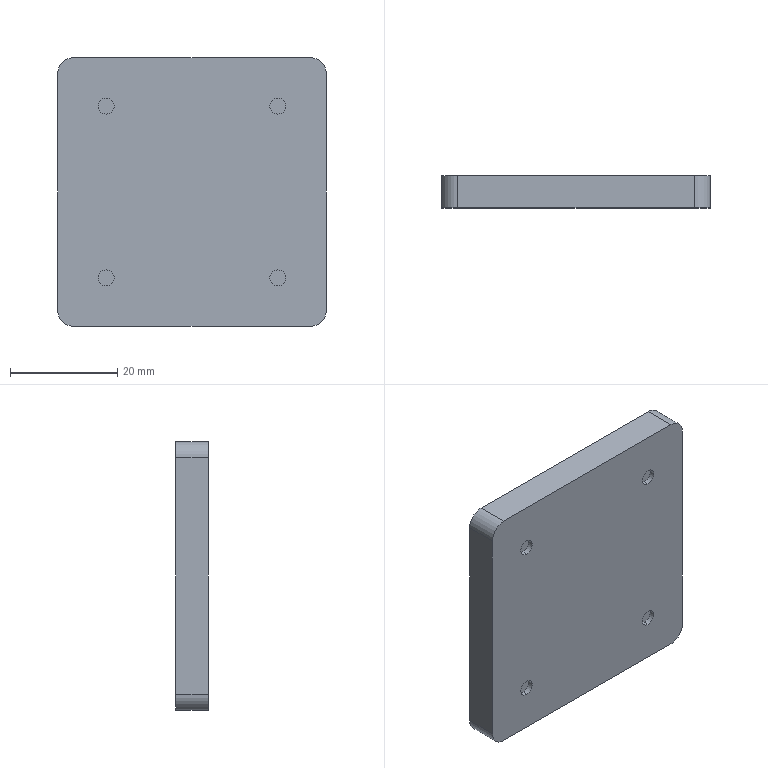Part | SolidWorks | features ICE 4, Extrusion 1, Fillet 1 | 1 solid | 28 faces | box 50 x 6 x 50 mm | volume 9918 mm3 | cylinder 16 | plane 12 | commonest cylinder face diameters 3 x10 6 x4 46 x2
STEP:
#1=CARTESIAN_POINT('',(16.,5.,17.5));
#2=VERTEX_POINT('',#1);
#3=CARTESIAN_POINT('',(16.,5.,14.5));
#4=VERTEX_POINT('',#3);
#5=CARTESIAN_POINT('',(16.,5.,16.));
#6=DIRECTION('',(0.,-1.,0.));
#7=DIRECTION('',(0.,0.,-1.));
#8=AXIS2_PLACEMENT_3D('',#5,#6,#7);
#9=CIRCLE('',#8,1.5);
#10=EDGE_CURVE('',#2,#4,#9,.T.);
#11=ORIENTED_EDGE('',*,*,#10,.F.);
#12=CARTESIAN_POINT('',(16.,4.,17.5));
#13=VERTEX_POINT('',#12);
#14=CARTESIAN_POINT('',(16.,5.,17.5));
#15=DIRECTION('',(0.,-1.,0.));
#16=VECTOR('',#15,1000.);
#17=LINE('',#14,#16);
#18=EDGE_CURVE('',#2,#13,#17,.T.);
#19=ORIENTED_EDGE('',*,*,#18,.T.);
#20=CARTESIAN_POINT('',(16.,4.,14.5));
#21=VERTEX_POINT('',#20);
#22=CARTESIAN_POINT('',(16.,4.,16.));
#23=DIRECTION('',(0.,-1.,0.));
#24=DIRECTION('',(0.,0.,-1.));
#25=AXIS2_PLACEMENT_3D('',#22,#23,#24);
#26=CIRCLE('',#25,1.5);
#27=EDGE_CURVE('',#13,#21,#26,.T.);
#28=ORIENTED_EDGE('',*,*,#27,.T.);
#29=CARTESIAN_POINT('',(16.,5.,14.5));
#30=DIRECTION('',(0.,-1.,0.));
#31=VECTOR('',#30,1000.);
#32=LINE('',#29,#31);
#33=EDGE_CURVE('',#4,#21,#32,.T.);
#34=ORIENTED_EDGE('',*,*,#33,.F.);
#35=EDGE_LOOP('',(#11,#19,#28,#34));
#36=FACE_OUTER_BOUND('',#35,.T.);
#37=CARTESIAN_POINT('',(16.,5.,16.));
#38=DIRECTION('',(0.,-1.,0.));
#39=DIRECTION('',(0.,0.,-1.));
#40=AXIS2_PLACEMENT_3D('',#37,#38,#39);
#41=CYLINDRICAL_SURFACE('',#40,1.5);
#42=ADVANCED_FACE('',(#36),#41,.F.);
#43=CARTESIAN_POINT('',(-16.,5.,-14.5));
#44=VERTEX_POINT('',#43);
#45=CARTESIAN_POINT('',(-16.,5.,-17.5));
#46=VERTEX_POINT('',#45);
#47=CARTESIAN_POINT('',(-16.,5.,-16.));
#48=DIRECTION('',(0.,-1.,0.));
#49=DIRECTION('',(0.,0.,-1.));
#50=AXIS2_PLACEMENT_3D('',#47,#48,#49);
#51=CIRCLE('',#50,1.5);
#52=EDGE_CURVE('',#44,#46,#51,.T.);
#53=ORIENTED_EDGE('',*,*,#52,.F.);
#54=CARTESIAN_POINT('',(-16.,4.,-14.5));
#55=VERTEX_POINT('',#54);
#56=CARTESIAN_POINT('',(-16.,5.,-14.5));
#57=DIRECTION('',(0.,-1.,0.));
#58=VECTOR('',#57,1000.);
#59=LINE('',#56,#58);
#60=EDGE_CURVE('',#44,#55,#59,.T.);
#61=ORIENTED_EDGE('',*,*,#60,.T.);
#62=CARTESIAN_POINT('',(-16.,4.,-17.5));
#63=VERTEX_POINT('',#62);
#64=CARTESIAN_POINT('',(-16.,4.,-16.));
#65=DIRECTION('',(0.,-1.,0.));
#66=DIRECTION('',(0.,0.,-1.));
#67=AXIS2_PLACEMENT_3D('',#64,#65,#66);
#68=CIRCLE('',#67,1.5);
#69=EDGE_CURVE('',#55,#63,#68,.T.);
#70=ORIENTED_EDGE('',*,*,#69,.T.);
#71=CARTESIAN_POINT('',(-16.,5.,-17.5));
#72=DIRECTION('',(0.,-1.,0.));
#73=VECTOR('',#72,1000.);
#74=LINE('',#71,#73);
#75=EDGE_CURVE('',#46,#63,#74,.T.);
#76=ORIENTED_EDGE('',*,*,#75,.F.);
#77=EDGE_LOOP('',(#53,#61,#70,#76));
#78=FACE_OUTER_BOUND('',#77,.T.);
#79=CARTESIAN_POINT('',(-16.,5.,-16.));
#80=DIRECTION('',(0.,-1.,0.));
#81=DIRECTION('',(0.,0.,-1.));
#82=AXIS2_PLACEMENT_3D('',#79,#80,#81);
#83=CYLINDRICAL_SURFACE('',#82,1.5);
#84=ADVANCED_FACE('',(#78),#83,.F.);
#85=CARTESIAN_POINT('',(16.,5.,-14.5));
#86=VERTEX_POINT('',#85);
#87=CARTESIAN_POINT('',(16.,5.,-17.5));
#88=VERTEX_POINT('',#87);
#89=CARTESIAN_POINT('',(16.,5.,-16.));
#90=DIRECTION('',(0.,-1.,0.));
#91=DIRECTION('',(0.,0.,-1.));
#92=AXIS2_PLACEMENT_3D('',#89,#90,#91);
#93=CIRCLE('',#92,1.5);
#94=EDGE_CURVE('',#86,#88,#93,.T.);
#95=ORIENTED_EDGE('',*,*,#94,.F.);
#96=CARTESIAN_POINT('',(16.,4.,-14.5));
#97=VERTEX_POINT('',#96);
#98=CARTESIAN_POINT('',(16.,5.,-14.5));
#99=DIRECTION('',(0.,-1.,0.));
#100=VECTOR('',#99,1000.);
#101=LINE('',#98,#100);
#102=EDGE_CURVE('',#86,#97,#101,.T.);
#103=ORIENTED_EDGE('',*,*,#102,.T.);
#104=CARTESIAN_POINT('',(16.,4.,-17.5));
#105=VERTEX_POINT('',#104);
#106=CARTESIAN_POINT('',(16.,4.,-16.));
#107=DIRECTION('',(0.,-1.,0.));
#108=DIRECTION('',(0.,0.,-1.));
#109=AXIS2_PLACEMENT_3D('',#106,#107,#108);
#110=CIRCLE('',#109,1.5);
#111=EDGE_CURVE('',#97,#105,#110,.T.);
#112=ORIENTED_EDGE('',*,*,#111,.T.);
#113=CARTESIAN_POINT('',(16.,5.,-17.5));
#114=DIRECTION('',(0.,-1.,0.));
#115=VECTOR('',#114,1000.);
#116=LINE('',#113,#115);
#117=EDGE_CURVE('',#88,#105,#116,.T.);
#118=ORIENTED_EDGE('',*,*,#117,.F.);
#119=EDGE_LOOP('',(#95,#103,#112,#118));
#120=FACE_OUTER_BOUND('',#119,.T.);
#121=CARTESIAN_POINT('',(16.,5.,-16.));
#122=DIRECTION('',(0.,-1.,0.));
#123=DIRECTION('',(0.,0.,-1.));
#124=AXIS2_PLACEMENT_3D('',#121,#122,#123);
#125=CYLINDRICAL_SURFACE('',#124,1.5);
#126=ADVANCED_FACE('',(#120),#125,.F.);
#127=CARTESIAN_POINT('',(-16.,5.,17.5));
#128=VERTEX_POINT('',#127);
#129=CARTESIAN_POINT('',(-16.,5.,14.5));
#130=VERTEX_POINT('',#129);
#131=CARTESIAN_POINT('',(-16.,5.,16.));
#132=DIRECTION('',(0.,-1.,0.));
#133=DIRECTION('',(0.,0.,-1.));
#134=AXIS2_PLACEMENT_3D('',#131,#132,#133);
#135=CIRCLE('',#134,1.5);
#136=EDGE_CURVE('',#128,#130,#135,.T.);
#137=ORIENTED_EDGE('',*,*,#136,.F.);
#138=CARTESIAN_POINT('',(-16.,4.,17.5));
#139=VERTEX_POINT('',#138);
#140=CARTESIAN_POINT('',(-16.,5.,17.5));
#141=DIRECTION('',(0.,-1.,0.));
#142=VECTOR('',#141,1000.);
#143=LINE('',#140,#142);
#144=EDGE_CURVE('',#128,#139,#143,.T.);
#145=ORIENTED_EDGE('',*,*,#144,.T.);
#146=CARTESIAN_POINT('',(-16.,4.,14.5));
#147=VERTEX_POINT('',#146);
#148=CARTESIAN_POINT('',(-16.,4.,16.));
#149=DIRECTION('',(0.,-1.,0.));
#150=DIRECTION('',(0.,0.,-1.));
#151=AXIS2_PLACEMENT_3D('',#148,#149,#150);
#152=CIRCLE('',#151,1.5);
#153=EDGE_CURVE('',#139,#147,#152,.T.);
#154=ORIENTED_EDGE('',*,*,#153,.T.);
#155=CARTESIAN_POINT('',(-16.,5.,14.5));
#156=DIRECTION('',(0.,-1.,0.));
#157=VECTOR('',#156,1000.);
#158=LINE('',#155,#157);
#159=EDGE_CURVE('',#130,#147,#158,.T.);
#160=ORIENTED_EDGE('',*,*,#159,.F.);
#161=EDGE_LOOP('',(#137,#145,#154,#160));
#162=FACE_OUTER_BOUND('',#161,.T.);
#163=CARTESIAN_POINT('',(-16.,5.,16.));
#164=DIRECTION('',(0.,-1.,0.));
#165=DIRECTION('',(0.,0.,-1.));
#166=AXIS2_PLACEMENT_3D('',#163,#164,#165);
#167=CYLINDRICAL_SURFACE('',#166,1.5);
#168=ADVANCED_FACE('',(#162),#167,.F.);
#169=CARTESIAN_POINT('',(20.,7.,18.5));
#170=VERTEX_POINT('',#169);
#171=CARTESIAN_POINT('',(20.,7.,21.5));
#172=VERTEX_POINT('',#171);
#173=CARTESIAN_POINT('',(20.,7.,20.));
#174=DIRECTION('',(0.,1.,0.));
#175=DIRECTION('',(0.,0.,1.));
#176=AXIS2_PLACEMENT_3D('',#173,#174,#175);
#177=CIRCLE('',#176,1.5);
#178=EDGE_CURVE('',#170,#172,#177,.T.);
#179=ORIENTED_EDGE('',*,*,#178,.F.);
#180=CARTESIAN_POINT('',(20.,10.,18.5));
#181=VERTEX_POINT('',#180);
#182=CARTESIAN_POINT('',(20.,7.,18.5));
#183=DIRECTION('',(0.,1.,0.));
#184=VECTOR('',#183,1000.);
#185=LINE('',#182,#184);
#186=EDGE_CURVE('',#170,#181,#185,.T.);
#187=ORIENTED_EDGE('',*,*,#186,.T.);
#188=CARTESIAN_POINT('',(20.,10.,21.5));
#189=VERTEX_POINT('',#188);
#190=CARTESIAN_POINT('',(20.,10.,20.));
#191=DIRECTION('',(0.,1.,0.));
#192=DIRECTION('',(0.,0.,1.));
#193=AXIS2_PLACEMENT_3D('',#190,#191,#192);
#194=CIRCLE('',#193,1.5);
#195=EDGE_CURVE('',#181,#189,#194,.T.);
#196=ORIENTED_EDGE('',*,*,#195,.T.);
#197=CARTESIAN_POINT('',(20.,7.,21.5));
#198=DIRECTION('',(0.,1.,0.));
#199=VECTOR('',#198,1000.);
#200=LINE('',#197,#199);
#201=EDGE_CURVE('',#172,#189,#200,.T.);
#202=ORIENTED_EDGE('',*,*,#201,.F.);
#203=EDGE_LOOP('',(#179,#187,#196,#202));
#204=FACE_OUTER_BOUND('',#203,.T.);
#205=CARTESIAN_POINT('',(20.,7.,20.));
#206=DIRECTION('',(0.,1.,0.));
#207=DIRECTION('',(0.,0.,1.));
#208=AXIS2_PLACEMENT_3D('',#205,#206,#207);
#209=CYLINDRICAL_SURFACE('',#208,1.5);
#210=ADVANCED_FACE('',(#204),#209,.F.);
#211=CARTESIAN_POINT('',(0.,7.,-23.));
#212=VERTEX_POINT('',#211);
#213=CARTESIAN_POINT('',(0.,7.,23.));
#214=VERTEX_POINT('',#213);
#215=CARTESIAN_POINT('',(0.,7.,0.));
#216=DIRECTION('',(0.,1.,0.));
#217=DIRECTION('',(0.,0.,1.));
#218=AXIS2_PLACEMENT_3D('',#215,#216,#217);
#219=CIRCLE('',#218,23.);
#220=EDGE_CURVE('',#212,#214,#219,.T.);
#221=ORIENTED_EDGE('',*,*,#220,.F.);
#222=CARTESIAN_POINT('',(0.,10.,-23.));
#223=VERTEX_POINT('',#222);
#224=CARTESIAN_POINT('',(0.,7.,-23.));
#225=DIRECTION('',(0.,1.,0.));
#226=VECTOR('',#225,1000.);
#227=LINE('',#224,#226);
#228=EDGE_CURVE('',#212,#223,#227,.T.);
#229=ORIENTED_EDGE('',*,*,#228,.T.);
#230=CARTESIAN_POINT('',(0.,10.,23.));
#231=VERTEX_POINT('',#230);
#232=CARTESIAN_POINT('',(0.,10.,0.));
#233=DIRECTION('',(0.,1.,0.));
#234=DIRECTION('',(0.,0.,1.));
#235=AXIS2_PLACEMENT_3D('',#232,#233,#234);
#236=CIRCLE('',#235,23.);
#237=EDGE_CURVE('',#223,#231,#236,.T.);
#238=ORIENTED_EDGE('',*,*,#237,.T.);
#239=CARTESIAN_POINT('',(0.,7.,23.));
#240=DIRECTION('',(0.,1.,0.));
#241=VECTOR('',#240,1000.);
#242=LINE('',#239,#241);
#243=EDGE_CURVE('',#214,#231,#242,.T.);
#244=ORIENTED_EDGE('',*,*,#243,.F.);
#245=EDGE_LOOP('',(#221,#229,#238,#244));
#246=FACE_OUTER_BOUND('',#245,.T.);
#247=CARTESIAN_POINT('',(0.,7.,0.));
#248=DIRECTION('',(0.,1.,0.));
#249=DIRECTION('',(0.,0.,1.));
#250=AXIS2_PLACEMENT_3D('',#247,#248,#249);
#251=CYLINDRICAL_SURFACE('',#250,23.);
#252=ADVANCED_FACE('',(#246),#251,.F.);
#253=CARTESIAN_POINT('',(25.,4.,-22.));
#254=VERTEX_POINT('',#253);
#255=CARTESIAN_POINT('',(25.,4.,22.));
#256=VERTEX_POINT('',#255);
#257=CARTESIAN_POINT('',(25.,4.,-51.));
#258=DIRECTION('',(0.,0.,1.));
#259=VECTOR('',#258,1000.);
#260=LINE('',#257,#259);
#261=EDGE_CURVE('',#254,#256,#260,.T.);
#262=ORIENTED_EDGE('',*,*,#261,.F.);
#263=CARTESIAN_POINT('',(25.,10.,-22.));
#264=VERTEX_POINT('',#263);
#265=CARTESIAN_POINT('',(25.,10.,-22.));
#266=DIRECTION('',(0.,1.,0.));
#267=VECTOR('',#266,1000.);
#268=LINE('',#265,#267);
#269=EDGE_CURVE('',#254,#264,#268,.T.);
#270=ORIENTED_EDGE('',*,*,#269,.T.);
#271=CARTESIAN_POINT('',(25.,10.,22.));
#272=VERTEX_POINT('',#271);
#273=CARTESIAN_POINT('',(25.,10.,25.));
#274=DIRECTION('',(0.,0.,-1.));
#275=VECTOR('',#274,1000.);
#276=LINE('',#273,#275);
#277=EDGE_CURVE('',#272,#264,#276,.T.);
#278=ORIENTED_EDGE('',*,*,#277,.F.);
#279=CARTESIAN_POINT('',(25.,10.,22.));
#280=DIRECTION('',(0.,-1.,0.));
#281=VECTOR('',#280,1000.);
#282=LINE('',#279,#281);
#283=EDGE_CURVE('',#272,#256,#282,.T.);
#284=ORIENTED_EDGE('',*,*,#283,.T.);
#285=EDGE_LOOP('',(#262,#270,#278,#284));
#286=FACE_OUTER_BOUND('',#285,.T.);
#287=CARTESIAN_POINT('',(25.,10.,25.));
#288=DIRECTION('',(-1.,0.,0.));
#289=DIRECTION('',(0.,0.,1.));
#290=AXIS2_PLACEMENT_3D('',#287,#288,#289);
#291=PLANE('',#290);
#292=ADVANCED_FACE('',(#286),#291,.F.);
#293=CARTESIAN_POINT('',(22.,4.,-25.));
#294=VERTEX_POINT('',#293);
#295=CARTESIAN_POINT('',(-22.,4.,-25.));
#296=VERTEX_POINT('',#295);
#297=CARTESIAN_POINT('',(-25.,4.,-25.));
#298=DIRECTION('',(-1.,0.,0.));
#299=VECTOR('',#298,1000.);
#300=LINE('',#297,#299);
#301=EDGE_CURVE('',#294,#296,#300,.T.);
#302=ORIENTED_EDGE('',*,*,#301,.T.);
#303=CARTESIAN_POINT('',(-22.,10.,-25.));
#304=VERTEX_POINT('',#303);
#305=CARTESIAN_POINT('',(-22.,10.,-25.));
#306=DIRECTION('',(0.,1.,0.));
#307=VECTOR('',#306,1000.);
#308=LINE('',#305,#307);
#309=EDGE_CURVE('',#296,#304,#308,.T.);
#310=ORIENTED_EDGE('',*,*,#309,.T.);
#311=CARTESIAN_POINT('',(22.,10.,-25.));
#312=VERTEX_POINT('',#311);
#313=CARTESIAN_POINT('',(-25.,10.,-25.));
#314=DIRECTION('',(-1.,0.,0.));
#315=VECTOR('',#314,1000.);
#316=LINE('',#313,#315);
#317=EDGE_CURVE('',#312,#304,#316,.T.);
#318=ORIENTED_EDGE('',*,*,#317,.F.);
#319=CARTESIAN_POINT('',(22.,10.,-25.));
#320=DIRECTION('',(0.,-1.,0.));
#321=VECTOR('',#320,1000.);
#322=LINE('',#319,#321);
#323=EDGE_CURVE('',#312,#294,#322,.T.);
#324=ORIENTED_EDGE('',*,*,#323,.T.);
#325=EDGE_LOOP('',(#302,#310,#318,#324));
#326=FACE_OUTER_BOUND('',#325,.T.);
#327=CARTESIAN_POINT('',(-25.,10.,-25.));
#328=DIRECTION('',(0.,0.,1.));
#329=DIRECTION('',(1.,0.,0.));
#330=AXIS2_PLACEMENT_3D('',#327,#328,#329);
#331=PLANE('',#330);
#332=ADVANCED_FACE('',(#326),#331,.F.);
#333=CARTESIAN_POINT('',(-25.,10.,-22.));
#334=VERTEX_POINT('',#333);
#335=CARTESIAN_POINT('',(-25.,10.,22.));
#336=VERTEX_POINT('',#335);
#337=CARTESIAN_POINT('',(-25.,10.,25.));
#338=DIRECTION('',(0.,0.,1.));
#339=VECTOR('',#338,1000.);
#340=LINE('',#337,#339);
#341=EDGE_CURVE('',#334,#336,#340,.T.);
#342=ORIENTED_EDGE('',*,*,#341,.F.);
#343=CARTESIAN_POINT('',(-25.,4.,-22.));
#344=VERTEX_POINT('',#343);
#345=CARTESIAN_POINT('',(-25.,10.,-22.));
#346=DIRECTION('',(0.,-1.,0.));
#347=VECTOR('',#346,1000.);
#348=LINE('',#345,#347);
#349=EDGE_CURVE('',#334,#344,#348,.T.);
#350=ORIENTED_EDGE('',*,*,#349,.T.);
#351=CARTESIAN_POINT('',(-25.,4.,22.));
#352=VERTEX_POINT('',#351);
#353=CARTESIAN_POINT('',(-25.,4.,-51.));
#354=DIRECTION('',(0.,0.,1.));
#355=VECTOR('',#354,1000.);
#356=LINE('',#353,#355);
#357=EDGE_CURVE('',#344,#352,#356,.T.);
#358=ORIENTED_EDGE('',*,*,#357,.T.);
#359=CARTESIAN_POINT('',(-25.,10.,22.));
#360=DIRECTION('',(0.,1.,0.));
#361=VECTOR('',#360,1000.);
#362=LINE('',#359,#361);
#363=EDGE_CURVE('',#352,#336,#362,.T.);
#364=ORIENTED_EDGE('',*,*,#363,.T.);
#365=EDGE_LOOP('',(#342,#350,#358,#364));
#366=FACE_OUTER_BOUND('',#365,.T.);
#367=CARTESIAN_POINT('',(-25.,10.,25.));
#368=DIRECTION('',(1.,0.,0.));
#369=DIRECTION('',(0.,0.,-1.));
#370=AXIS2_PLACEMENT_3D('',#367,#368,#369);
#371=PLANE('',#370);
#372=ADVANCED_FACE('',(#366),#371,.F.);
#373=CARTESIAN_POINT('',(22.,4.,25.));
#374=VERTEX_POINT('',#373);
#375=CARTESIAN_POINT('',(-22.,4.,25.));
#376=VERTEX_POINT('',#375);
#377=CARTESIAN_POINT('',(-25.,4.,25.));
#378=DIRECTION('',(-1.,0.,0.));
#379=VECTOR('',#378,1000.);
#380=LINE('',#377,#379);
#381=EDGE_CURVE('',#374,#376,#380,.T.);
#382=ORIENTED_EDGE('',*,*,#381,.F.);
#383=CARTESIAN_POINT('',(22.,10.,25.));
#384=VERTEX_POINT('',#383);
#385=CARTESIAN_POINT('',(22.,10.,25.));
#386=DIRECTION('',(0.,1.,0.));
#387=VECTOR('',#386,1000.);
#388=LINE('',#385,#387);
#389=EDGE_CURVE('',#374,#384,#388,.T.);
#390=ORIENTED_EDGE('',*,*,#389,.T.);
#391=CARTESIAN_POINT('',(-22.,10.,25.));
#392=VERTEX_POINT('',#391);
#393=CARTESIAN_POINT('',(-25.,10.,25.));
#394=DIRECTION('',(1.,0.,0.));
#395=VECTOR('',#394,1000.);
#396=LINE('',#393,#395);
#397=EDGE_CURVE('',#392,#384,#396,.T.);
#398=ORIENTED_EDGE('',*,*,#397,.F.);
#399=CARTESIAN_POINT('',(-22.,10.,25.));
#400=DIRECTION('',(0.,-1.,0.));
#401=VECTOR('',#400,1000.);
#402=LINE('',#399,#401);
#403=EDGE_CURVE('',#392,#376,#402,.T.);
#404=ORIENTED_EDGE('',*,*,#403,.T.);
#405=EDGE_LOOP('',(#382,#390,#398,#404));
#406=FACE_OUTER_BOUND('',#405,.T.);
#407=CARTESIAN_POINT('',(-25.,10.,25.));
#408=DIRECTION('',(0.,0.,-1.));
#409=DIRECTION('',(-1.,0.,0.));
#410=AXIS2_PLACEMENT_3D('',#407,#408,#409);
#411=PLANE('',#410);
#412=ADVANCED_FACE('',(#406),#411,.F.);
#413=CARTESIAN_POINT('',(20.,10.,20.));
#414=DIRECTION('',(0.,1.,0.));
#415=DIRECTION('',(0.,0.,1.));
#416=AXIS2_PLACEMENT_3D('',#413,#414,#415);
#417=CIRCLE('',#416,1.5);
#418=EDGE_CURVE('',#189,#181,#417,.T.);
#419=ORIENTED_EDGE('',*,*,#418,.F.);
#420=ORIENTED_EDGE('',*,*,#195,.F.);
#421=EDGE_LOOP('',(#419,#420));
#422=FACE_BOUND('',#421,.T.);
#423=CARTESIAN_POINT('',(0.,10.,0.));
#424=DIRECTION('',(0.,1.,0.));
#425=DIRECTION('',(0.,0.,1.));
#426=AXIS2_PLACEMENT_3D('',#423,#424,#425);
#427=CIRCLE('',#426,23.);
#428=EDGE_CURVE('',#231,#223,#427,.T.);
#429=ORIENTED_EDGE('',*,*,#428,.F.);
#430=ORIENTED_EDGE('',*,*,#237,.F.);
#431=EDGE_LOOP('',(#429,#430));
#432=FACE_BOUND('',#431,.T.);
#433=ORIENTED_EDGE('',*,*,#317,.T.);
#434=CARTESIAN_POINT('',(-22.,10.,-22.));
#435=DIRECTION('',(0.,1.,0.));
#436=DIRECTION('',(0.,0.,-1.));
#437=AXIS2_PLACEMENT_3D('',#434,#435,#436);
#438=CIRCLE('',#437,3.);
#439=EDGE_CURVE('',#304,#334,#438,.T.);
#440=ORIENTED_EDGE('',*,*,#439,.T.);
#441=ORIENTED_EDGE('',*,*,#341,.T.);
#442=CARTESIAN_POINT('',(-22.,10.,22.));
#443=DIRECTION('',(0.,1.,0.));
#444=DIRECTION('',(0.,0.,-1.));
#445=AXIS2_PLACEMENT_3D('',#442,#443,#444);
#446=CIRCLE('',#445,3.);
#447=EDGE_CURVE('',#336,#392,#446,.T.);
#448=ORIENTED_EDGE('',*,*,#447,.T.);
#449=ORIENTED_EDGE('',*,*,#397,.T.);
#450=CARTESIAN_POINT('',(22.,10.,22.));
#451=DIRECTION('',(0.,1.,0.));
#452=DIRECTION('',(0.,0.,-1.));
#453=AXIS2_PLACEMENT_3D('',#450,#451,#452);
#454=CIRCLE('',#453,3.);
#455=EDGE_CURVE('',#384,#272,#454,.T.);
#456=ORIENTED_EDGE('',*,*,#455,.T.);
#457=ORIENTED_EDGE('',*,*,#277,.T.);
#458=CARTESIAN_POINT('',(22.,10.,-22.));
#459=DIRECTION('',(0.,1.,0.));
#460=DIRECTION('',(0.,0.,-1.));
#461=AXIS2_PLACEMENT_3D('',#458,#459,#460);
#462=CIRCLE('',#461,3.);
#463=EDGE_CURVE('',#264,#312,#462,.T.);
#464=ORIENTED_EDGE('',*,*,#463,.T.);
#465=EDGE_LOOP('',(#433,#440,#441,#448,#449,#456,#457,#464));
#466=FACE_OUTER_BOUND('',#465,.T.);
#467=CARTESIAN_POINT('',(0.,10.,0.));
#468=DIRECTION('',(0.,-1.,0.));
#469=DIRECTION('',(0.,0.,-1.));
#470=AXIS2_PLACEMENT_3D('',#467,#468,#469);
#471=PLANE('',#470);
#472=ADVANCED_FACE('',(#422,#432,#466),#471,.F.);
#473=ORIENTED_EDGE('',*,*,#228,.F.);
#474=CARTESIAN_POINT('',(0.,7.,0.));
#475=DIRECTION('',(0.,1.,0.));
#476=DIRECTION('',(0.,0.,1.));
#477=AXIS2_PLACEMENT_3D('',#474,#475,#476);
#478=CIRCLE('',#477,23.);
#479=EDGE_CURVE('',#214,#212,#478,.T.);
#480=ORIENTED_EDGE('',*,*,#479,.F.);
#481=ORIENTED_EDGE('',*,*,#243,.T.);
#482=ORIENTED_EDGE('',*,*,#428,.T.);
#483=EDGE_LOOP('',(#473,#480,#481,#482));
#484=FACE_OUTER_BOUND('',#483,.T.);
#485=CARTESIAN_POINT('',(0.,7.,0.));
#486=DIRECTION('',(0.,1.,0.));
#487=DIRECTION('',(0.,0.,1.));
#488=AXIS2_PLACEMENT_3D('',#485,#486,#487);
#489=CYLINDRICAL_SURFACE('',#488,23.);
#490=ADVANCED_FACE('',(#484),#489,.F.);
#491=ORIENTED_EDGE('',*,*,#479,.T.);
#492=ORIENTED_EDGE('',*,*,#220,.T.);
#493=EDGE_LOOP('',(#491,#492));
#494=FACE_OUTER_BOUND('',#493,.T.);
#495=CARTESIAN_POINT('',(0.,7.,0.));
#496=DIRECTION('',(0.,1.,0.));
#497=DIRECTION('',(0.,0.,1.));
#498=AXIS2_PLACEMENT_3D('',#495,#496,#497);
#499=PLANE('',#498);
#500=ADVANCED_FACE('',(#494),#499,.T.);
#501=ORIENTED_EDGE('',*,*,#186,.F.);
#502=CARTESIAN_POINT('',(20.,7.,20.));
#503=DIRECTION('',(0.,1.,0.));
#504=DIRECTION('',(0.,0.,1.));
#505=AXIS2_PLACEMENT_3D('',#502,#503,#504);
#506=CIRCLE('',#505,1.5);
#507=EDGE_CURVE('',#172,#170,#506,.T.);
#508=ORIENTED_EDGE('',*,*,#507,.F.);
#509=ORIENTED_EDGE('',*,*,#201,.T.);
#510=ORIENTED_EDGE('',*,*,#418,.T.);
#511=EDGE_LOOP('',(#501,#508,#509,#510));
#512=FACE_OUTER_BOUND('',#511,.T.);
#513=CARTESIAN_POINT('',(20.,7.,20.));
#514=DIRECTION('',(0.,1.,0.));
#515=DIRECTION('',(0.,0.,1.));
#516=AXIS2_PLACEMENT_3D('',#513,#514,#515);
#517=CYLINDRICAL_SURFACE('',#516,1.5);
#518=ADVANCED_FACE('',(#512),#517,.F.);
#519=ORIENTED_EDGE('',*,*,#507,.T.);
#520=ORIENTED_EDGE('',*,*,#178,.T.);
#521=EDGE_LOOP('',(#519,#520));
#522=FACE_OUTER_BOUND('',#521,.T.);
#523=CARTESIAN_POINT('',(20.,7.,20.));
#524=DIRECTION('',(0.,1.,0.));
#525=DIRECTION('',(0.,0.,1.));
#526=AXIS2_PLACEMENT_3D('',#523,#524,#525);
#527=PLANE('',#526);
#528=ADVANCED_FACE('',(#522),#527,.T.);
#529=CARTESIAN_POINT('',(16.,4.,16.));
#530=DIRECTION('',(0.,-1.,0.));
#531=DIRECTION('',(0.,0.,-1.));
#532=AXIS2_PLACEMENT_3D('',#529,#530,#531);
#533=CIRCLE('',#532,1.5);
#534=EDGE_CURVE('',#21,#13,#533,.T.);
#535=ORIENTED_EDGE('',*,*,#534,.F.);
#536=ORIENTED_EDGE('',*,*,#27,.F.);
#537=EDGE_LOOP('',(#535,#536));
#538=FACE_BOUND('',#537,.T.);
#539=CARTESIAN_POINT('',(-16.,4.,-16.));
#540=DIRECTION('',(0.,-1.,0.));
#541=DIRECTION('',(0.,0.,-1.));
#542=AXIS2_PLACEMENT_3D('',#539,#540,#541);
#543=CIRCLE('',#542,1.5);
#544=EDGE_CURVE('',#63,#55,#543,.T.);
#545=ORIENTED_EDGE('',*,*,#544,.F.);
#546=ORIENTED_EDGE('',*,*,#69,.F.);
#547=EDGE_LOOP('',(#545,#546));
#548=FACE_BOUND('',#547,.T.);
#549=CARTESIAN_POINT('',(16.,4.,-16.));
#550=DIRECTION('',(0.,-1.,0.));
#551=DIRECTION('',(0.,0.,-1.));
#552=AXIS2_PLACEMENT_3D('',#549,#550,#551);
#553=CIRCLE('',#552,1.5);
#554=EDGE_CURVE('',#105,#97,#553,.T.);
#555=ORIENTED_EDGE('',*,*,#554,.F.);
#556=ORIENTED_EDGE('',*,*,#111,.F.);
#557=EDGE_LOOP('',(#555,#556));
#558=FACE_BOUND('',#557,.T.);
#559=CARTESIAN_POINT('',(-16.,4.,16.));
#560=DIRECTION('',(0.,-1.,0.));
#561=DIRECTION('',(0.,0.,-1.));
#562=AXIS2_PLACEMENT_3D('',#559,#560,#561);
#563=CIRCLE('',#562,1.5);
#564=EDGE_CURVE('',#147,#139,#563,.T.);
#565=ORIENTED_EDGE('',*,*,#564,.F.);
#566=ORIENTED_EDGE('',*,*,#153,.F.);
#567=EDGE_LOOP('',(#565,#566));
#568=FACE_BOUND('',#567,.T.);
#569=ORIENTED_EDGE('',*,*,#357,.F.);
#570=CARTESIAN_POINT('',(-22.,4.,-22.));
#571=DIRECTION('',(0.,-1.,0.));
#572=DIRECTION('',(0.,0.,1.));
#573=AXIS2_PLACEMENT_3D('',#570,#571,#572);
#574=CIRCLE('',#573,3.);
#575=EDGE_CURVE('',#344,#296,#574,.T.);
#576=ORIENTED_EDGE('',*,*,#575,.T.);
#577=ORIENTED_EDGE('',*,*,#301,.F.);
#578=CARTESIAN_POINT('',(22.,4.,-22.));
#579=DIRECTION('',(0.,-1.,0.));
#580=DIRECTION('',(0.,0.,1.));
#581=AXIS2_PLACEMENT_3D('',#578,#579,#580);
#582=CIRCLE('',#581,3.);
#583=EDGE_CURVE('',#294,#254,#582,.T.);
#584=ORIENTED_EDGE('',*,*,#583,.T.);
#585=ORIENTED_EDGE('',*,*,#261,.T.);
#586=CARTESIAN_POINT('',(22.,4.,22.));
#587=DIRECTION('',(0.,-1.,0.));
#588=DIRECTION('',(0.,0.,1.));
#589=AXIS2_PLACEMENT_3D('',#586,#587,#588);
#590=CIRCLE('',#589,3.);
#591=EDGE_CURVE('',#256,#374,#590,.T.);
#592=ORIENTED_EDGE('',*,*,#591,.T.);
#593=ORIENTED_EDGE('',*,*,#381,.T.);
#594=CARTESIAN_POINT('',(-22.,4.,22.));
#595=DIRECTION('',(0.,-1.,0.));
#596=DIRECTION('',(0.,0.,1.));
#597=AXIS2_PLACEMENT_3D('',#594,#595,#596);
#598=CIRCLE('',#597,3.);
#599=EDGE_CURVE('',#376,#352,#598,.T.);
#600=ORIENTED_EDGE('',*,*,#599,.T.);
#601=EDGE_LOOP('',(#569,#576,#577,#584,#585,#592,#593,#600));
#602=FACE_OUTER_BOUND('',#601,.T.);
#603=CARTESIAN_POINT('',(-25.,4.,-51.));
#604=DIRECTION('',(0.,1.,0.));
#605=DIRECTION('',(0.,0.,1.));
#606=AXIS2_PLACEMENT_3D('',#603,#604,#605);
#607=PLANE('',#606);
#608=ADVANCED_FACE('',(#538,#548,#558,#568,#602),#607,.F.);
#609=ORIENTED_EDGE('',*,*,#439,.F.);
#610=ORIENTED_EDGE('',*,*,#309,.F.);
#611=ORIENTED_EDGE('',*,*,#575,.F.);
#612=ORIENTED_EDGE('',*,*,#349,.F.);
#613=EDGE_LOOP('',(#609,#610,#611,#612));
#614=FACE_OUTER_BOUND('',#613,.T.);
#615=CARTESIAN_POINT('',(-22.,10.,-22.));
#616=DIRECTION('',(0.,-1.,0.));
#617=DIRECTION('',(0.,0.,-1.));
#618=AXIS2_PLACEMENT_3D('',#615,#616,#617);
#619=CYLINDRICAL_SURFACE('',#618,3.);
#620=ADVANCED_FACE('',(#614),#619,.T.);
#621=ORIENTED_EDGE('',*,*,#463,.F.);
#622=ORIENTED_EDGE('',*,*,#269,.F.);
#623=ORIENTED_EDGE('',*,*,#583,.F.);
#624=ORIENTED_EDGE('',*,*,#323,.F.);
#625=EDGE_LOOP('',(#621,#622,#623,#624));
#626=FACE_OUTER_BOUND('',#625,.T.);
#627=CARTESIAN_POINT('',(22.,10.,-22.));
#628=DIRECTION('',(0.,-1.,0.));
#629=DIRECTION('',(0.,0.,-1.));
#630=AXIS2_PLACEMENT_3D('',#627,#628,#629);
#631=CYLINDRICAL_SURFACE('',#630,3.);
#632=ADVANCED_FACE('',(#626),#631,.T.);
#633=ORIENTED_EDGE('',*,*,#455,.F.);
#634=ORIENTED_EDGE('',*,*,#389,.F.);
#635=ORIENTED_EDGE('',*,*,#591,.F.);
#636=ORIENTED_EDGE('',*,*,#283,.F.);
#637=EDGE_LOOP('',(#633,#634,#635,#636));
#638=FACE_OUTER_BOUND('',#637,.T.);
#639=CARTESIAN_POINT('',(22.,10.,22.));
#640=DIRECTION('',(0.,-1.,0.));
#641=DIRECTION('',(0.,0.,-1.));
#642=AXIS2_PLACEMENT_3D('',#639,#640,#641);
#643=CYLINDRICAL_SURFACE('',#642,3.);
#644=ADVANCED_FACE('',(#638),#643,.T.);
#645=ORIENTED_EDGE('',*,*,#447,.F.);
#646=ORIENTED_EDGE('',*,*,#363,.F.);
#647=ORIENTED_EDGE('',*,*,#599,.F.);
#648=ORIENTED_EDGE('',*,*,#403,.F.);
#649=EDGE_LOOP('',(#645,#646,#647,#648));
#650=FACE_OUTER_BOUND('',#649,.T.);
#651=CARTESIAN_POINT('',(-22.,10.,22.));
#652=DIRECTION('',(0.,-1.,0.));
#653=DIRECTION('',(0.,0.,-1.));
#654=AXIS2_PLACEMENT_3D('',#651,#652,#653);
#655=CYLINDRICAL_SURFACE('',#654,3.);
#656=ADVANCED_FACE('',(#650),#655,.T.);
#657=ORIENTED_EDGE('',*,*,#144,.F.);
#658=CARTESIAN_POINT('',(-16.,5.,16.));
#659=DIRECTION('',(0.,-1.,0.));
#660=DIRECTION('',(0.,0.,-1.));
#661=AXIS2_PLACEMENT_3D('',#658,#659,#660);
#662=CIRCLE('',#661,1.5);
#663=EDGE_CURVE('',#130,#128,#662,.T.);
#664=ORIENTED_EDGE('',*,*,#663,.F.);
#665=ORIENTED_EDGE('',*,*,#159,.T.);
#666=ORIENTED_EDGE('',*,*,#564,.T.);
#667=EDGE_LOOP('',(#657,#664,#665,#666));
#668=FACE_OUTER_BOUND('',#667,.T.);
#669=CARTESIAN_POINT('',(-16.,5.,16.));
#670=DIRECTION('',(0.,-1.,0.));
#671=DIRECTION('',(0.,0.,-1.));
#672=AXIS2_PLACEMENT_3D('',#669,#670,#671);
#673=CYLINDRICAL_SURFACE('',#672,1.5);
#674=ADVANCED_FACE('',(#668),#673,.F.);
#675=ORIENTED_EDGE('',*,*,#663,.T.);
#676=ORIENTED_EDGE('',*,*,#136,.T.);
#677=EDGE_LOOP('',(#675,#676));
#678=FACE_OUTER_BOUND('',#677,.T.);
#679=CARTESIAN_POINT('',(-16.,5.,16.));
#680=DIRECTION('',(0.,-1.,0.));
#681=DIRECTION('',(0.,0.,-1.));
#682=AXIS2_PLACEMENT_3D('',#679,#680,#681);
#683=PLANE('',#682);
#684=ADVANCED_FACE('',(#678),#683,.T.);
#685=ORIENTED_EDGE('',*,*,#102,.F.);
#686=CARTESIAN_POINT('',(16.,5.,-16.));
#687=DIRECTION('',(0.,-1.,0.));
#688=DIRECTION('',(0.,0.,-1.));
#689=AXIS2_PLACEMENT_3D('',#686,#687,#688);
#690=CIRCLE('',#689,1.5);
#691=EDGE_CURVE('',#88,#86,#690,.T.);
#692=ORIENTED_EDGE('',*,*,#691,.F.);
#693=ORIENTED_EDGE('',*,*,#117,.T.);
#694=ORIENTED_EDGE('',*,*,#554,.T.);
#695=EDGE_LOOP('',(#685,#692,#693,#694));
#696=FACE_OUTER_BOUND('',#695,.T.);
#697=CARTESIAN_POINT('',(16.,5.,-16.));
#698=DIRECTION('',(0.,-1.,0.));
#699=DIRECTION('',(0.,0.,-1.));
#700=AXIS2_PLACEMENT_3D('',#697,#698,#699);
#701=CYLINDRICAL_SURFACE('',#700,1.5);
#702=ADVANCED_FACE('',(#696),#701,.F.);
#703=ORIENTED_EDGE('',*,*,#691,.T.);
#704=ORIENTED_EDGE('',*,*,#94,.T.);
#705=EDGE_LOOP('',(#703,#704));
#706=FACE_OUTER_BOUND('',#705,.T.);
#707=CARTESIAN_POINT('',(16.,5.,-16.));
#708=DIRECTION('',(0.,-1.,0.));
#709=DIRECTION('',(0.,0.,-1.));
#710=AXIS2_PLACEMENT_3D('',#707,#708,#709);
#711=PLANE('',#710);
#712=ADVANCED_FACE('',(#706),#711,.T.);
#713=ORIENTED_EDGE('',*,*,#60,.F.);
#714=CARTESIAN_POINT('',(-16.,5.,-16.));
#715=DIRECTION('',(0.,-1.,0.));
#716=DIRECTION('',(0.,0.,-1.));
#717=AXIS2_PLACEMENT_3D('',#714,#715,#716);
#718=CIRCLE('',#717,1.5);
#719=EDGE_CURVE('',#46,#44,#718,.T.);
#720=ORIENTED_EDGE('',*,*,#719,.F.);
#721=ORIENTED_EDGE('',*,*,#75,.T.);
#722=ORIENTED_EDGE('',*,*,#544,.T.);
#723=EDGE_LOOP('',(#713,#720,#721,#722));
#724=FACE_OUTER_BOUND('',#723,.T.);
#725=CARTESIAN_POINT('',(-16.,5.,-16.));
#726=DIRECTION('',(0.,-1.,0.));
#727=DIRECTION('',(0.,0.,-1.));
#728=AXIS2_PLACEMENT_3D('',#725,#726,#727);
#729=CYLINDRICAL_SURFACE('',#728,1.5);
#730=ADVANCED_FACE('',(#724),#729,.F.);
#731=ORIENTED_EDGE('',*,*,#719,.T.);
#732=ORIENTED_EDGE('',*,*,#52,.T.);
#733=EDGE_LOOP('',(#731,#732));
#734=FACE_OUTER_BOUND('',#733,.T.);
#735=CARTESIAN_POINT('',(-16.,5.,-16.));
#736=DIRECTION('',(0.,-1.,0.));
#737=DIRECTION('',(0.,0.,-1.));
#738=AXIS2_PLACEMENT_3D('',#735,#736,#737);
#739=PLANE('',#738);
#740=ADVANCED_FACE('',(#734),#739,.T.);
#741=ORIENTED_EDGE('',*,*,#18,.F.);
#742=CARTESIAN_POINT('',(16.,5.,16.));
#743=DIRECTION('',(0.,-1.,0.));
#744=DIRECTION('',(0.,0.,-1.));
#745=AXIS2_PLACEMENT_3D('',#742,#743,#744);
#746=CIRCLE('',#745,1.5);
#747=EDGE_CURVE('',#4,#2,#746,.T.);
#748=ORIENTED_EDGE('',*,*,#747,.F.);
#749=ORIENTED_EDGE('',*,*,#33,.T.);
#750=ORIENTED_EDGE('',*,*,#534,.T.);
#751=EDGE_LOOP('',(#741,#748,#749,#750));
#752=FACE_OUTER_BOUND('',#751,.T.);
#753=CARTESIAN_POINT('',(16.,5.,16.));
#754=DIRECTION('',(0.,-1.,0.));
#755=DIRECTION('',(0.,0.,-1.));
#756=AXIS2_PLACEMENT_3D('',#753,#754,#755);
#757=CYLINDRICAL_SURFACE('',#756,1.5);
#758=ADVANCED_FACE('',(#752),#757,.F.);
#759=ORIENTED_EDGE('',*,*,#747,.T.);
#760=ORIENTED_EDGE('',*,*,#10,.T.);
#761=EDGE_LOOP('',(#759,#760));
#762=FACE_OUTER_BOUND('',#761,.T.);
#763=CARTESIAN_POINT('',(16.,5.,16.));
#764=DIRECTION('',(0.,-1.,0.));
#765=DIRECTION('',(0.,0.,-1.));
#766=AXIS2_PLACEMENT_3D('',#763,#764,#765);
#767=PLANE('',#766);
#768=ADVANCED_FACE('',(#762),#767,.T.);
#769=CLOSED_SHELL('',(#42,#84,#126,#168,#210,#252,#292,#332,#372,#412,#472,#490,#500,#518,#528,#608,#620,#632,#644,#656,#674,#684,#702,#712,#730,#740,#758,#768));
#770=MANIFOLD_SOLID_BREP('',#769);
#771=CARTESIAN_POINT('',(0.,0.,0.));
#772=DIRECTION('',(0.,0.,1.));
#773=DIRECTION('',(1.,0.,0.));
#774=AXIS2_PLACEMENT_3D('',#771,#772,#773);
#775=(LENGTH_UNIT()NAMED_UNIT(*)SI_UNIT(.MILLI.,.METRE.));
#776=UNCERTAINTY_MEASURE_WITH_UNIT(LENGTH_MEASURE(0.00001),#775,'','');
#777=(NAMED_UNIT(*)PLANE_ANGLE_UNIT()SI_UNIT($,.RADIAN.));
#778=(NAMED_UNIT(*)SI_UNIT($,.STERADIAN.)SOLID_ANGLE_UNIT());
#779=(GEOMETRIC_REPRESENTATION_CONTEXT(3)GLOBAL_UNCERTAINTY_ASSIGNED_CONTEXT((#776))GLOBAL_UNIT_ASSIGNED_CONTEXT((#775,#777,#778))REPRESENTATION_CONTEXT('',''));
#780=ADVANCED_BREP_SHAPE_REPRESENTATION('',(#770,#774),#779);